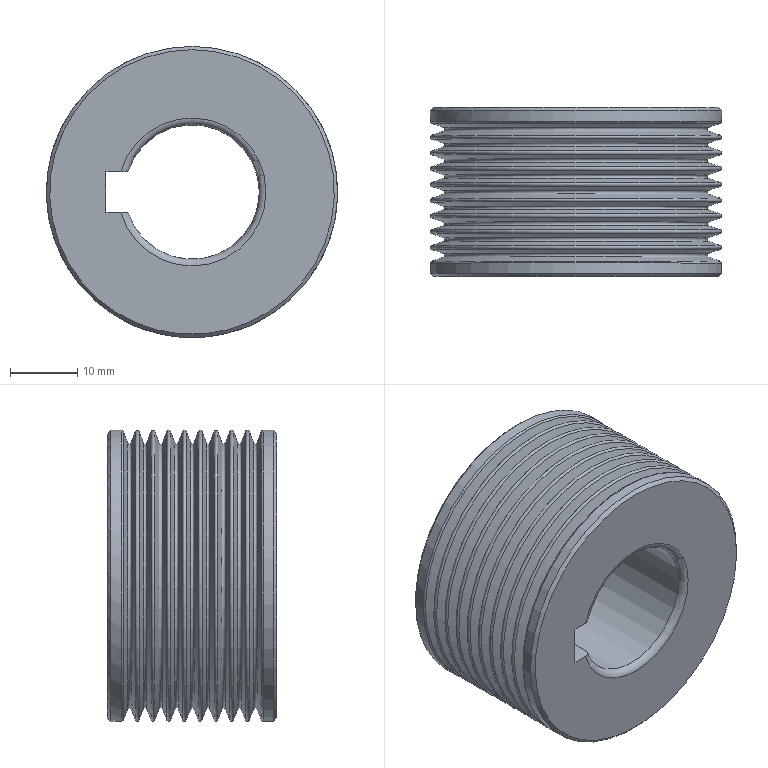Part | STEP file | Roller 9 ribbed 2 | 1 solid | 49 faces | box 43.308 x 25.164 x 43.308 mm | volume 25808 mm3 | torus 21 | cone 20 | plane 5 | cylinder 3 | commonest cylinder face diameters 20 x1 43.3 x1 43.308 x1